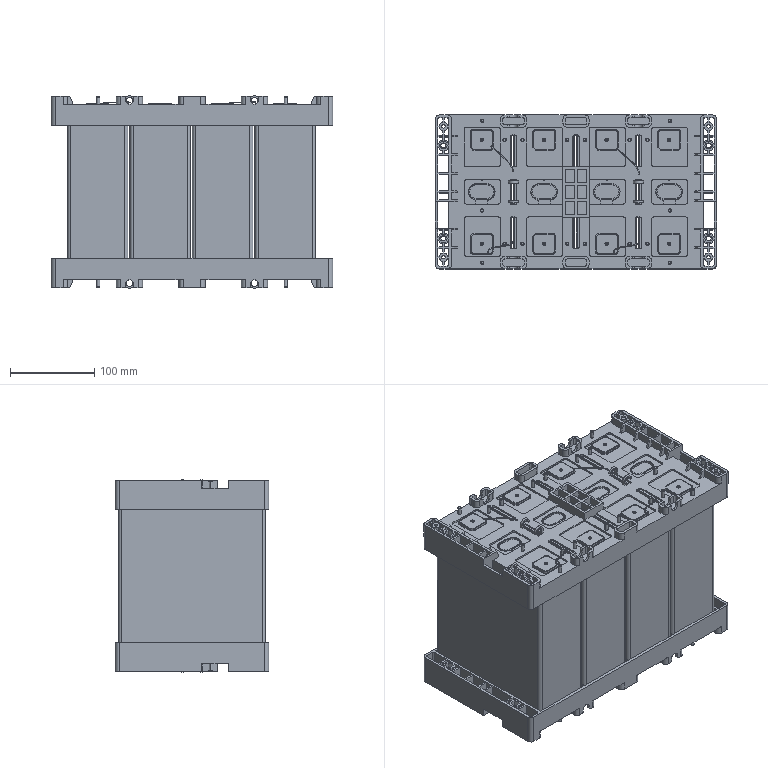Part | NX | features BREP 10 | 10 solids | 2672 faces | box 333 x 182 x 227.965 mm | volume 10643125 mm3 | plane 1736 | cylinder 784 | cone 120 | spline 24 | torus 8 | commonest cylinder face diameters 4 x224 6 x216 10 x108 2 x48 8 x32 4.22 x24